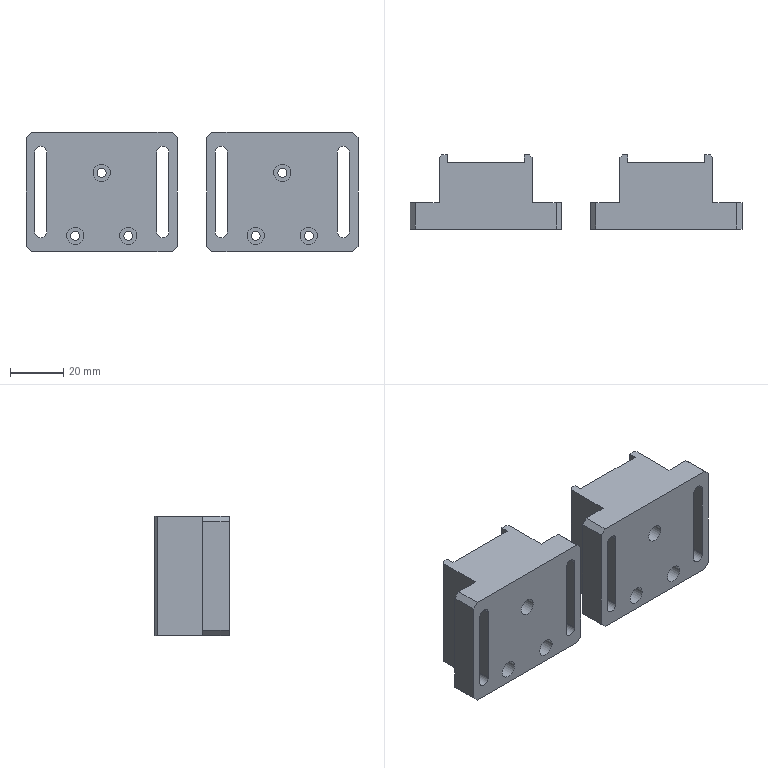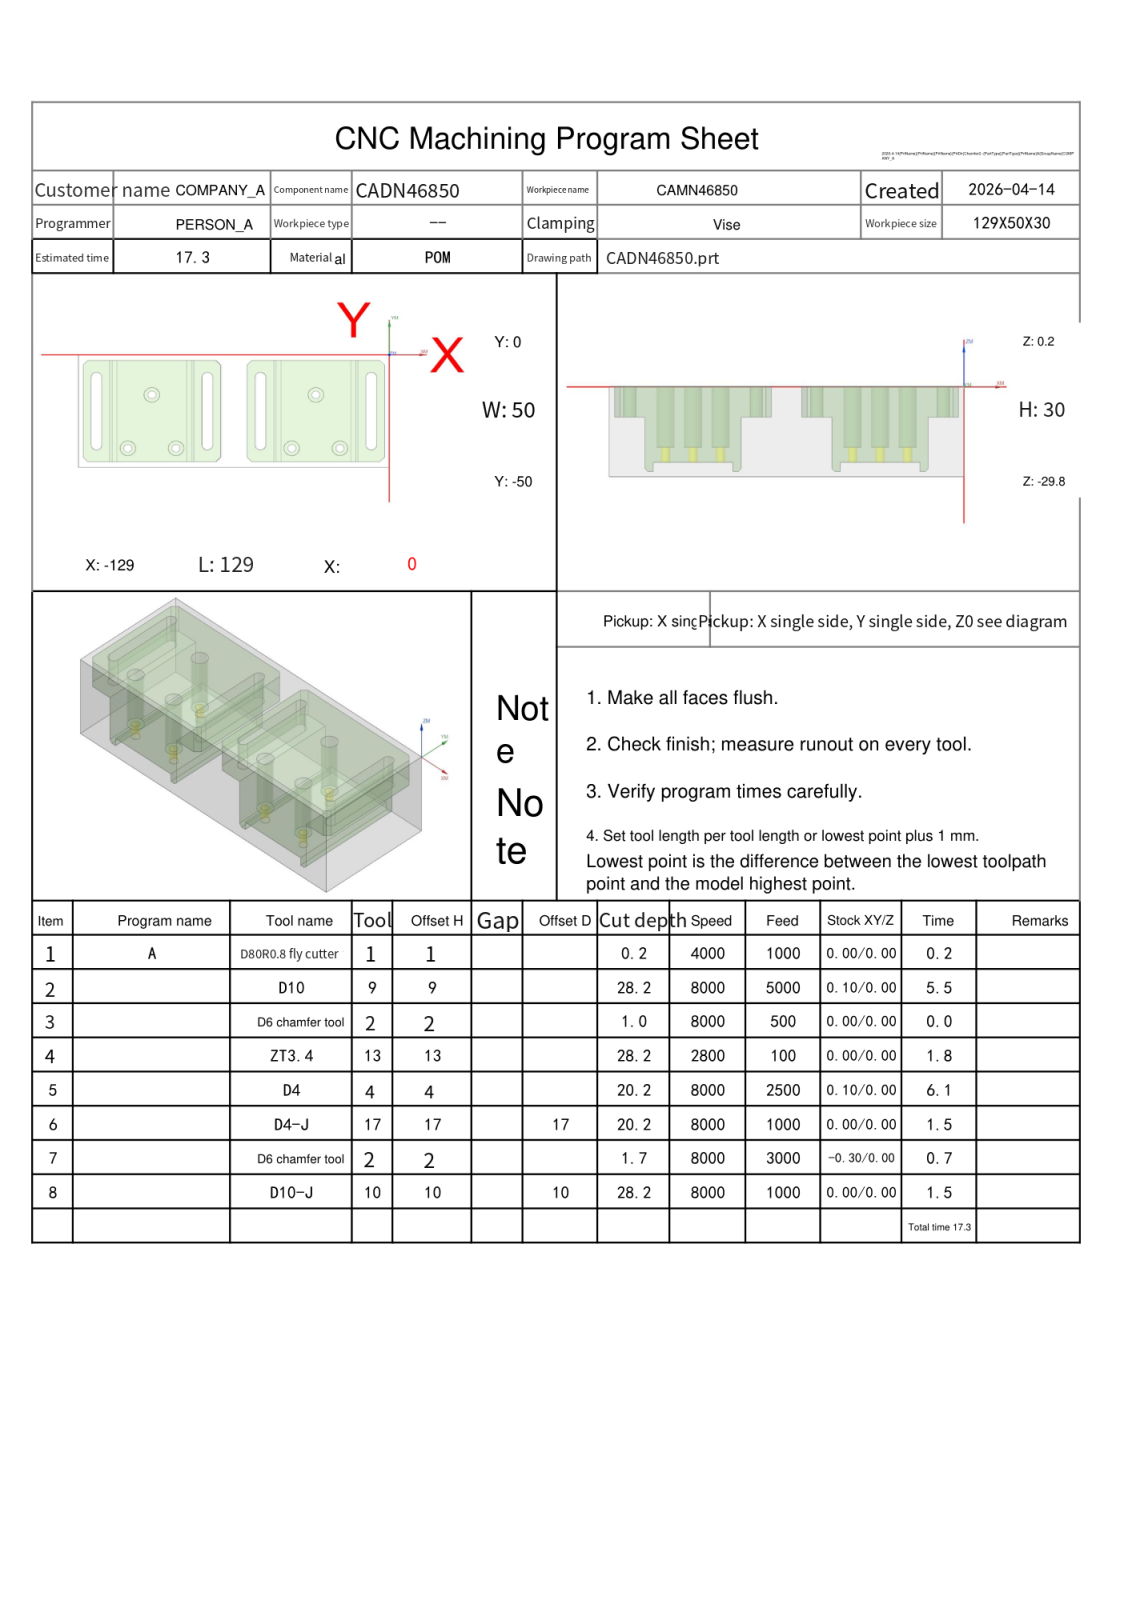NC program | NX | posted by the shop | part box 125 x 28 x 45 mm
Lines 1997 to 3630 of 4607, first 1124 of 1634 lines:
N5 T04 M06
(D4  D=4. R=0. H=04 ce=0.10 di=0.10)
G00 G90 G54 X-7.65 Y-25. M03 S6000
G43 H04 Z20.
M08
Z.5
G01 Y-40. Z.44 F2500.
G03 X-7.5 Y-40.15 Z.439 I.15 J0.0
X-7.35 Y-40. Z.438 I0.0 J.15
G01 Y-10. Z.318
G03 X-7.5 Y-9.85 Z.317 I-.15 J0.0
X-7.65 Y-10. Z.316 I0.0 J-.15
G01 Y-40. Z.195
G03 X-7.5 Y-40.15 Z.194 I.15 J0.0
X-7.35 Y-40. Z.194 I0.0 J.15
G01 Y-10. Z.073
G03 X-7.5 Y-9.85 Z.072 I-.15 J0.0
X-7.65 Y-10. Z.071 I0.0 J-.15
G01 Y-40. Z-.049
G03 X-7.5 Y-40.15 Z-.05 I.15 J0.0
X-7.35 Y-40. Z-.051 I0.0 J.15
G01 Y-10. Z-.171
G03 X-7.5 Y-9.85 Z-.172 I-.15 J0.0
X-7.65 Y-10. Z-.173 I0.0 J-.15
G01 Y-40. Z-.294
G03 X-7.5 Y-40.15 Z-.294 I.15 J0.0
X-7.35 Y-40. Z-.295 I0.0 J.15
G01 Y-10. Z-.416
G03 X-7.5 Y-9.85 Z-.417 I-.15 J0.0
X-7.65 Y-10. Z-.418 I0.0 J-.15
G01 Y-40. Z-.538
G03 X-7.5 Y-40.15 Z-.539 I.15 J0.0
X-7.35 Y-40. Z-.54 I0.0 J.15
G01 Y-10. Z-.66
G03 X-7.5 Y-9.85 Z-.661 I-.15 J0.0
X-7.65 Y-10. Z-.662 I0.0 J-.15
G01 Y-40. Z-.782
G03 X-7.5 Y-40.15 Z-.783 I.15 J0.0
X-7.35 Y-40. Z-.784 I0.0 J.15
G01 Y-10. Z-.905
G03 X-7.5 Y-9.85 Z-.906 I-.15 J0.0
X-7.65 Y-10. Z-.907 I0.0 J-.15
G01 Y-40. Z-1.027
G03 X-7.5 Y-40.15 Z-1.028 I.15 J0.0
X-7.35 Y-40. Z-1.029 I0.0 J.15
G01 Y-10. Z-1.149
G03 X-7.5 Y-9.85 Z-1.15 I-.15 J0.0
X-7.65 Y-10. Z-1.151 I0.0 J-.15
G01 Y-40. Z-1.271
G03 X-7.5 Y-40.15 Z-1.272 I.15 J0.0
X-7.35 Y-40. Z-1.273 I0.0 J.15
G01 Y-10. Z-1.394
G03 X-7.5 Y-9.85 Z-1.394 I-.15 J0.0
X-7.65 Y-10. Z-1.395 I0.0 J-.15
G01 Y-40. Z-1.516
G03 X-7.5 Y-40.15 Z-1.517 I.15 J0.0
X-7.35 Y-40. Z-1.518 I0.0 J.15
G01 Y-10. Z-1.638
G03 X-7.5 Y-9.85 Z-1.639 I-.15 J0.0
X-7.65 Y-10. Z-1.64 I0.0 J-.15
G01 Y-40. Z-1.76
G03 X-7.5 Y-40.15 Z-1.761 I.15 J0.0
X-7.35 Y-40. Z-1.762 I0.0 J.15
G01 Y-10. Z-1.882
G03 X-7.5 Y-9.85 Z-1.883 I-.15 J0.0
X-7.65 Y-10. Z-1.884 I0.0 J-.15
G01 Y-40. Z-2.005
G03 X-7.5 Y-40.15 Z-2.006 I.15 J0.0
X-7.35 Y-40. Z-2.007 I0.0 J.15
G01 Y-10. Z-2.127
G03 X-7.5 Y-9.85 Z-2.128 I-.15 J0.0
X-7.65 Y-10. Z-2.129 I0.0 J-.15
G01 Y-40. Z-2.249
G03 X-7.5 Y-40.15 Z-2.25 I.15 J0.0
X-7.35 Y-40. Z-2.251 I0.0 J.15
G01 Y-10. Z-2.371
G03 X-7.5 Y-9.85 Z-2.372 I-.15 J0.0
X-7.65 Y-10. Z-2.373 I0.0 J-.15
G01 Y-40. Z-2.494
G03 X-7.5 Y-40.15 Z-2.494 I.15 J0.0
X-7.35 Y-40. Z-2.495 I0.0 J.15
G01 Y-10. Z-2.616
G03 X-7.5 Y-9.85 Z-2.617 I-.15 J0.0
X-7.65 Y-10. Z-2.618 I0.0 J-.15
G01 Y-40. Z-2.738
G03 X-7.5 Y-40.15 Z-2.739 I.15 J0.0
X-7.35 Y-40. Z-2.74 I0.0 J.15
G01 Y-10. Z-2.86
G03 X-7.5 Y-9.85 Z-2.861 I-.15 J0.0
X-7.65 Y-10. Z-2.862 I0.0 J-.15
G01 Y-40. Z-2.982
G03 X-7.5 Y-40.15 Z-2.983 I.15 J0.0
X-7.35 Y-40. Z-2.984 I0.0 J.15
G01 Y-10. Z-3.105
G03 X-7.5 Y-9.85 Z-3.106 I-.15 J0.0
X-7.65 Y-10. Z-3.107 I0.0 J-.15
G01 Y-40. Z-3.227
G03 X-7.5 Y-40.15 Z-3.228 I.15 J0.0
X-7.35 Y-40. Z-3.229 I0.0 J.15
G01 Y-10. Z-3.349
G03 X-7.5 Y-9.85 Z-3.35 I-.15 J0.0
X-7.65 Y-10. Z-3.351 I0.0 J-.15
G01 Y-40. Z-3.471
G03 X-7.5 Y-40.15 Z-3.472 I.15 J0.0
X-7.35 Y-40. Z-3.473 I0.0 J.15
G01 Y-10. Z-3.594
G03 X-7.5 Y-9.85 Z-3.594 I-.15 J0.0
X-7.65 Y-10. Z-3.595 I0.0 J-.15
G01 Y-40. Z-3.716
G03 X-7.5 Y-40.15 Z-3.717 I.15 J0.0
X-7.35 Y-40. Z-3.718 I0.0 J.15
G01 Y-10. Z-3.838
G03 X-7.5 Y-9.85 Z-3.839 I-.15 J0.0
X-7.65 Y-10. Z-3.84 I0.0 J-.15
G01 Y-40. Z-3.96
G03 X-7.5 Y-40.15 Z-3.961 I.15 J0.0
X-7.35 Y-40. Z-3.962 I0.0 J.15
G01 Y-10. Z-4.082
G03 X-7.5 Y-9.85 Z-4.083 I-.15 J0.0
X-7.65 Y-10. Z-4.084 I0.0 J-.15
G01 Y-40. Z-4.205
G03 X-7.5 Y-40.15 Z-4.206 I.15 J0.0
X-7.35 Y-40. Z-4.207 I0.0 J.15
G01 Y-10. Z-4.327
G03 X-7.5 Y-9.85 Z-4.328 I-.15 J0.0
X-7.65 Y-10. Z-4.329 I0.0 J-.15
G01 Y-40. Z-4.449
G03 X-7.5 Y-40.15 Z-4.45 I.15 J0.0
X-7.35 Y-40. Z-4.451 I0.0 J.15
G01 Y-10. Z-4.571
G03 X-7.5 Y-9.85 Z-4.572 I-.15 J0.0
X-7.65 Y-10. Z-4.573 I0.0 J-.15
G01 Y-40. Z-4.694
G03 X-7.5 Y-40.15 Z-4.694 I.15 J0.0
X-7.35 Y-40. Z-4.695 I0.0 J.15
G01 Y-10. Z-4.816
G03 X-7.5 Y-9.85 Z-4.817 I-.15 J0.0
X-7.65 Y-10. Z-4.818 I0.0 J-.15
G01 Y-40. Z-4.938
G03 X-7.5 Y-40.15 Z-4.939 I.15 J0.0
X-7.35 Y-40. Z-4.94 I0.0 J.15
G01 Y-10. Z-5.06
G03 X-7.5 Y-9.85 Z-5.061 I-.15 J0.0
X-7.65 Y-10. Z-5.062 I0.0 J-.15
G01 Y-40. Z-5.182
G03 X-7.5 Y-40.15 Z-5.183 I.15 J0.0
X-7.35 Y-40. Z-5.184 I0.0 J.15
G01 Y-10. Z-5.305
G03 X-7.5 Y-9.85 Z-5.306 I-.15 J0.0
X-7.65 Y-10. Z-5.307 I0.0 J-.15
G01 Y-40. Z-5.427
G03 X-7.5 Y-40.15 Z-5.428 I.15 J0.0
X-7.35 Y-40. Z-5.429 I0.0 J.15
G01 Y-10. Z-5.549
G03 X-7.5 Y-9.85 Z-5.55 I-.15 J0.0
X-7.65 Y-10. Z-5.551 I0.0 J-.15
G01 Y-40. Z-5.671
G03 X-7.5 Y-40.15 Z-5.672 I.15 J0.0
X-7.35 Y-40. Z-5.673 I0.0 J.15
G01 Y-10. Z-5.794
G03 X-7.5 Y-9.85 Z-5.794 I-.15 J0.0
X-7.65 Y-10. Z-5.795 I0.0 J-.15
G01 Y-40. Z-5.916
G03 X-7.5 Y-40.15 Z-5.917 I.15 J0.0
X-7.35 Y-40. Z-5.918 I0.0 J.15
G01 Y-10. Z-6.038
G03 X-7.5 Y-9.85 Z-6.039 I-.15 J0.0
X-7.65 Y-10. Z-6.04 I0.0 J-.15
G01 Y-40. Z-6.16
G03 X-7.5 Y-40.15 Z-6.161 I.15 J0.0
X-7.35 Y-40. Z-6.162 I0.0 J.15
G01 Y-10. Z-6.282
G03 X-7.5 Y-9.85 Z-6.283 I-.15 J0.0
X-7.65 Y-10. Z-6.284 I0.0 J-.15
G01 Y-40. Z-6.405
G03 X-7.5 Y-40.15 Z-6.406 I.15 J0.0
X-7.35 Y-40. Z-6.407 I0.0 J.15
G01 Y-10. Z-6.527
G03 X-7.5 Y-9.85 Z-6.528 I-.15 J0.0
X-7.65 Y-10. Z-6.529 I0.0 J-.15
G01 Y-40. Z-6.649
G03 X-7.5 Y-40.15 Z-6.65 I.15 J0.0
X-7.35 Y-40. Z-6.651 I0.0 J.15
G01 Y-10. Z-6.771
G03 X-7.5 Y-9.85 Z-6.772 I-.15 J0.0
X-7.65 Y-10. Z-6.773 I0.0 J-.15
G01 Y-40. Z-6.894
G03 X-7.5 Y-40.15 Z-6.894 I.15 J0.0
X-7.35 Y-40. Z-6.895 I0.0 J.15
G01 Y-10. Z-7.016
G03 X-7.5 Y-9.85 Z-7.017 I-.15 J0.0
X-7.65 Y-10. Z-7.018 I0.0 J-.15
G01 Y-40. Z-7.138
G03 X-7.5 Y-40.15 Z-7.139 I.15 J0.0
X-7.35 Y-40. Z-7.14 I0.0 J.15
G01 Y-10. Z-7.26
G03 X-7.5 Y-9.85 Z-7.261 I-.15 J0.0
X-7.65 Y-10. Z-7.262 I0.0 J-.15
G01 Y-40. Z-7.382
G03 X-7.5 Y-40.15 Z-7.383 I.15 J0.0
X-7.35 Y-40. Z-7.384 I0.0 J.15
G01 Y-10. Z-7.505
G03 X-7.5 Y-9.85 Z-7.506 I-.15 J0.0
X-7.65 Y-10. Z-7.507 I0.0 J-.15
G01 Y-40. Z-7.627
G03 X-7.5 Y-40.15 Z-7.628 I.15 J0.0
X-7.35 Y-40. Z-7.629 I0.0 J.15
G01 Y-10. Z-7.749
G03 X-7.5 Y-9.85 Z-7.75 I-.15 J0.0
X-7.65 Y-10. Z-7.751 I0.0 J-.15
G01 Y-40. Z-7.871
G03 X-7.5 Y-40.15 Z-7.872 I.15 J0.0
X-7.35 Y-40. Z-7.873 I0.0 J.15
G01 Y-10. Z-7.994
G03 X-7.5 Y-9.85 Z-7.994 I-.15 J0.0
X-7.65 Y-10. Z-7.995 I0.0 J-.15
G01 Y-40. Z-8.116
G03 X-7.5 Y-40.15 Z-8.117 I.15 J0.0
X-7.35 Y-40. Z-8.118 I0.0 J.15
G01 Y-10. Z-8.238
G03 X-7.5 Y-9.85 Z-8.239 I-.15 J0.0
X-7.65 Y-10. Z-8.24 I0.0 J-.15
G01 Y-40. Z-8.36
G03 X-7.5 Y-40.15 Z-8.361 I.15 J0.0
X-7.35 Y-40. Z-8.362 I0.0 J.15
G01 Y-10. Z-8.482
G03 X-7.5 Y-9.85 Z-8.483 I-.15 J0.0
X-7.65 Y-10. Z-8.484 I0.0 J-.15
G01 Y-40. Z-8.605
G03 X-7.5 Y-40.15 Z-8.606 I.15 J0.0
X-7.35 Y-40. Z-8.607 I0.0 J.15
G01 Y-10. Z-8.727
G03 X-7.5 Y-9.85 Z-8.728 I-.15 J0.0
X-7.65 Y-10. Z-8.729 I0.0 J-.15
G01 Y-40. Z-8.849
G03 X-7.5 Y-40.15 Z-8.85 I.15 J0.0
X-7.35 Y-40. Z-8.851 I0.0 J.15
G01 Y-10. Z-8.971
G03 X-7.5 Y-9.85 Z-8.972 I-.15 J0.0
X-7.65 Y-10. Z-8.973 I0.0 J-.15
G01 Y-40. Z-9.094
G03 X-7.5 Y-40.15 Z-9.094 I.15 J0.0
X-7.35 Y-40. Z-9.095 I0.0 J.15
G01 Y-10. Z-9.216
G03 X-7.5 Y-9.85 Z-9.217 I-.15 J0.0
X-7.65 Y-10. Z-9.218 I0.0 J-.15
G01 Y-40. Z-9.338
G03 X-7.5 Y-40.15 Z-9.339 I.15 J0.0
X-7.35 Y-40. Z-9.34 I0.0 J.15
G01 Y-10. Z-9.46
G03 X-7.5 Y-9.85 Z-9.461 I-.15 J0.0
X-7.65 Y-10. Z-9.462 I0.0 J-.15
G01 Y-40. Z-9.582
G03 X-7.5 Y-40.15 Z-9.583 I.15 J0.0
X-7.35 Y-40. Z-9.584 I0.0 J.15
G01 Y-10. Z-9.705
G03 X-7.5 Y-9.85 Z-9.706 I-.15 J0.0
X-7.65 Y-10. Z-9.707 I0.0 J-.15
G01 Y-40. Z-9.827
G03 X-7.5 Y-40.15 Z-9.828 I.15 J0.0
X-7.35 Y-40. Z-9.829 I0.0 J.15
G01 Y-10. Z-9.949
G03 X-7.5 Y-9.85 Z-9.95 I-.15 J0.0
X-7.65 Y-10. Z-9.951 I0.0 J-.15
G01 Y-40. Z-10.071
G03 X-7.5 Y-40.15 Z-10.072 I.15 J0.0
X-7.35 Y-40. Z-10.073 I0.0 J.15
G01 Y-10. Z-10.194
G03 X-7.5 Y-9.85 Z-10.194 I-.15 J0.0
X-7.65 Y-10. Z-10.195 I0.0 J-.15
G01 Y-40. Z-10.316
G03 X-7.5 Y-40.15 Z-10.317 I.15 J0.0
X-7.35 Y-40. Z-10.318 I0.0 J.15
G01 Y-10. Z-10.438
G03 X-7.5 Y-9.85 Z-10.439 I-.15 J0.0
X-7.65 Y-10. Z-10.44 I0.0 J-.15
G01 Y-25. Z-10.5
Y-40.
G03 X-7.5 Y-40.15 I.15 J0.0
X-7.35 Y-40. I0.0 J.15
G01 Y-10.
G03 X-7.5 Y-9.85 I-.15 J0.0
X-7.65 Y-10. I0.0 J-.15
G01 Y-25.
Y-25.5
Z-9.5
G00 Z20.
X-53.35 Y-25.
Z.5
G01 Y-10. Z.44
G03 X-53.5 Y-9.85 Z.439 I-.15 J0.0
X-53.65 Y-10. Z.438 I0.0 J-.15
G01 Y-40. Z.318
G03 X-53.5 Y-40.15 Z.317 I.15 J0.0
X-53.35 Y-40. Z.316 I0.0 J.15
G01 Y-10. Z.195
G03 X-53.5 Y-9.85 Z.194 I-.15 J0.0
X-53.65 Y-10. Z.194 I0.0 J-.15
G01 Y-40. Z.073
G03 X-53.5 Y-40.15 Z.072 I.15 J0.0
X-53.35 Y-40. Z.071 I0.0 J.15
G01 Y-10. Z-.049
G03 X-53.5 Y-9.85 Z-.05 I-.15 J0.0
X-53.65 Y-10. Z-.051 I0.0 J-.15
G01 Y-40. Z-.171
G03 X-53.5 Y-40.15 Z-.172 I.15 J0.0
X-53.35 Y-40. Z-.173 I0.0 J.15
G01 Y-10. Z-.294
G03 X-53.5 Y-9.85 Z-.294 I-.15 J0.0
X-53.65 Y-10. Z-.295 I0.0 J-.15
G01 Y-40. Z-.416
G03 X-53.5 Y-40.15 Z-.417 I.15 J0.0
X-53.35 Y-40. Z-.418 I0.0 J.15
G01 Y-10. Z-.538
G03 X-53.5 Y-9.85 Z-.539 I-.15 J0.0
X-53.65 Y-10. Z-.54 I0.0 J-.15
G01 Y-40. Z-.66
G03 X-53.5 Y-40.15 Z-.661 I.15 J0.0
X-53.35 Y-40. Z-.662 I0.0 J.15
G01 Y-10. Z-.782
G03 X-53.5 Y-9.85 Z-.783 I-.15 J0.0
X-53.65 Y-10. Z-.784 I0.0 J-.15
G01 Y-40. Z-.905
G03 X-53.5 Y-40.15 Z-.906 I.15 J0.0
X-53.35 Y-40. Z-.907 I0.0 J.15
G01 Y-10. Z-1.027
G03 X-53.5 Y-9.85 Z-1.028 I-.15 J0.0
X-53.65 Y-10. Z-1.029 I0.0 J-.15
G01 Y-40. Z-1.149
G03 X-53.5 Y-40.15 Z-1.15 I.15 J0.0
X-53.35 Y-40. Z-1.151 I0.0 J.15
G01 Y-10. Z-1.271
G03 X-53.5 Y-9.85 Z-1.272 I-.15 J0.0
X-53.65 Y-10. Z-1.273 I0.0 J-.15
G01 Y-40. Z-1.394
G03 X-53.5 Y-40.15 Z-1.394 I.15 J0.0
X-53.35 Y-40. Z-1.395 I0.0 J.15
G01 Y-10. Z-1.516
G03 X-53.5 Y-9.85 Z-1.517 I-.15 J0.0
X-53.65 Y-10. Z-1.518 I0.0 J-.15
G01 Y-40. Z-1.638
G03 X-53.5 Y-40.15 Z-1.639 I.15 J0.0
X-53.35 Y-40. Z-1.64 I0.0 J.15
G01 Y-10. Z-1.76
G03 X-53.5 Y-9.85 Z-1.761 I-.15 J0.0
X-53.65 Y-10. Z-1.762 I0.0 J-.15
G01 Y-40. Z-1.882
G03 X-53.5 Y-40.15 Z-1.883 I.15 J0.0
X-53.35 Y-40. Z-1.884 I0.0 J.15
G01 Y-10. Z-2.005
G03 X-53.5 Y-9.85 Z-2.006 I-.15 J0.0
X-53.65 Y-10. Z-2.007 I0.0 J-.15
G01 Y-40. Z-2.127
G03 X-53.5 Y-40.15 Z-2.128 I.15 J0.0
X-53.35 Y-40. Z-2.129 I0.0 J.15
G01 Y-10. Z-2.249
G03 X-53.5 Y-9.85 Z-2.25 I-.15 J0.0
X-53.65 Y-10. Z-2.251 I0.0 J-.15
G01 Y-40. Z-2.371
G03 X-53.5 Y-40.15 Z-2.372 I.15 J0.0
X-53.35 Y-40. Z-2.373 I0.0 J.15
G01 Y-10. Z-2.494
G03 X-53.5 Y-9.85 Z-2.494 I-.15 J0.0
X-53.65 Y-10. Z-2.495 I0.0 J-.15
G01 Y-40. Z-2.616
G03 X-53.5 Y-40.15 Z-2.617 I.15 J0.0
X-53.35 Y-40. Z-2.618 I0.0 J.15
G01 Y-10. Z-2.738
G03 X-53.5 Y-9.85 Z-2.739 I-.15 J0.0
X-53.65 Y-10. Z-2.74 I0.0 J-.15
G01 Y-40. Z-2.86
G03 X-53.5 Y-40.15 Z-2.861 I.15 J0.0
X-53.35 Y-40. Z-2.862 I0.0 J.15
G01 Y-10. Z-2.982
G03 X-53.5 Y-9.85 Z-2.983 I-.15 J0.0
X-53.65 Y-10. Z-2.984 I0.0 J-.15
G01 Y-40. Z-3.105
G03 X-53.5 Y-40.15 Z-3.106 I.15 J0.0
X-53.35 Y-40. Z-3.107 I0.0 J.15
G01 Y-10. Z-3.227
G03 X-53.5 Y-9.85 Z-3.228 I-.15 J0.0
X-53.65 Y-10. Z-3.229 I0.0 J-.15
G01 Y-40. Z-3.349
G03 X-53.5 Y-40.15 Z-3.35 I.15 J0.0
X-53.35 Y-40. Z-3.351 I0.0 J.15
G01 Y-10. Z-3.471
G03 X-53.5 Y-9.85 Z-3.472 I-.15 J0.0
X-53.65 Y-10. Z-3.473 I0.0 J-.15
G01 Y-40. Z-3.594
G03 X-53.5 Y-40.15 Z-3.594 I.15 J0.0
X-53.35 Y-40. Z-3.595 I0.0 J.15
G01 Y-10. Z-3.716
G03 X-53.5 Y-9.85 Z-3.717 I-.15 J0.0
X-53.65 Y-10. Z-3.718 I0.0 J-.15
G01 Y-40. Z-3.838
G03 X-53.5 Y-40.15 Z-3.839 I.15 J0.0
X-53.35 Y-40. Z-3.84 I0.0 J.15
G01 Y-10. Z-3.96
G03 X-53.5 Y-9.85 Z-3.961 I-.15 J0.0
X-53.65 Y-10. Z-3.962 I0.0 J-.15
G01 Y-40. Z-4.082
G03 X-53.5 Y-40.15 Z-4.083 I.15 J0.0
X-53.35 Y-40. Z-4.084 I0.0 J.15
G01 Y-10. Z-4.205
G03 X-53.5 Y-9.85 Z-4.206 I-.15 J0.0
X-53.65 Y-10. Z-4.207 I0.0 J-.15
G01 Y-40. Z-4.327
G03 X-53.5 Y-40.15 Z-4.328 I.15 J0.0
X-53.35 Y-40. Z-4.329 I0.0 J.15
G01 Y-10. Z-4.449
G03 X-53.5 Y-9.85 Z-4.45 I-.15 J0.0
X-53.65 Y-10. Z-4.451 I0.0 J-.15
G01 Y-40. Z-4.571
G03 X-53.5 Y-40.15 Z-4.572 I.15 J0.0
X-53.35 Y-40. Z-4.573 I0.0 J.15
G01 Y-10. Z-4.694
G03 X-53.5 Y-9.85 Z-4.694 I-.15 J0.0
X-53.65 Y-10. Z-4.695 I0.0 J-.15
G01 Y-40. Z-4.816
G03 X-53.5 Y-40.15 Z-4.817 I.15 J0.0
X-53.35 Y-40. Z-4.818 I0.0 J.15
G01 Y-10. Z-4.938
G03 X-53.5 Y-9.85 Z-4.939 I-.15 J0.0
X-53.65 Y-10. Z-4.94 I0.0 J-.15
G01 Y-40. Z-5.06
G03 X-53.5 Y-40.15 Z-5.061 I.15 J0.0
X-53.35 Y-40. Z-5.062 I0.0 J.15
G01 Y-10. Z-5.182
G03 X-53.5 Y-9.85 Z-5.183 I-.15 J0.0
X-53.65 Y-10. Z-5.184 I0.0 J-.15
G01 Y-40. Z-5.305
G03 X-53.5 Y-40.15 Z-5.306 I.15 J0.0
X-53.35 Y-40. Z-5.307 I0.0 J.15
G01 Y-10. Z-5.427
G03 X-53.5 Y-9.85 Z-5.428 I-.15 J0.0
X-53.65 Y-10. Z-5.429 I0.0 J-.15
G01 Y-40. Z-5.549
G03 X-53.5 Y-40.15 Z-5.55 I.15 J0.0
X-53.35 Y-40. Z-5.551 I0.0 J.15
G01 Y-10. Z-5.671
G03 X-53.5 Y-9.85 Z-5.672 I-.15 J0.0
X-53.65 Y-10. Z-5.673 I0.0 J-.15
G01 Y-40. Z-5.794
G03 X-53.5 Y-40.15 Z-5.794 I.15 J0.0
X-53.35 Y-40. Z-5.795 I0.0 J.15
G01 Y-10. Z-5.916
G03 X-53.5 Y-9.85 Z-5.917 I-.15 J0.0
X-53.65 Y-10. Z-5.918 I0.0 J-.15
G01 Y-40. Z-6.038
G03 X-53.5 Y-40.15 Z-6.039 I.15 J0.0
X-53.35 Y-40. Z-6.04 I0.0 J.15
G01 Y-10. Z-6.16
G03 X-53.5 Y-9.85 Z-6.161 I-.15 J0.0
X-53.65 Y-10. Z-6.162 I0.0 J-.15
G01 Y-40. Z-6.282
G03 X-53.5 Y-40.15 Z-6.283 I.15 J0.0
X-53.35 Y-40. Z-6.284 I0.0 J.15
G01 Y-10. Z-6.405
G03 X-53.5 Y-9.85 Z-6.406 I-.15 J0.0
X-53.65 Y-10. Z-6.407 I0.0 J-.15
G01 Y-40. Z-6.527
G03 X-53.5 Y-40.15 Z-6.528 I.15 J0.0
X-53.35 Y-40. Z-6.529 I0.0 J.15
G01 Y-10. Z-6.649
G03 X-53.5 Y-9.85 Z-6.65 I-.15 J0.0
X-53.65 Y-10. Z-6.651 I0.0 J-.15
G01 Y-40. Z-6.771
G03 X-53.5 Y-40.15 Z-6.772 I.15 J0.0
X-53.35 Y-40. Z-6.773 I0.0 J.15
G01 Y-10. Z-6.894
G03 X-53.5 Y-9.85 Z-6.894 I-.15 J0.0
X-53.65 Y-10. Z-6.895 I0.0 J-.15
G01 Y-40. Z-7.016
G03 X-53.5 Y-40.15 Z-7.017 I.15 J0.0
X-53.35 Y-40. Z-7.018 I0.0 J.15
G01 Y-10. Z-7.138
G03 X-53.5 Y-9.85 Z-7.139 I-.15 J0.0
X-53.65 Y-10. Z-7.14 I0.0 J-.15
G01 Y-40. Z-7.26
G03 X-53.5 Y-40.15 Z-7.261 I.15 J0.0
X-53.35 Y-40. Z-7.262 I0.0 J.15
G01 Y-10. Z-7.382
G03 X-53.5 Y-9.85 Z-7.383 I-.15 J0.0
X-53.65 Y-10. Z-7.384 I0.0 J-.15
G01 Y-40. Z-7.505
G03 X-53.5 Y-40.15 Z-7.506 I.15 J0.0
X-53.35 Y-40. Z-7.507 I0.0 J.15
G01 Y-10. Z-7.627
G03 X-53.5 Y-9.85 Z-7.628 I-.15 J0.0
X-53.65 Y-10. Z-7.629 I0.0 J-.15
G01 Y-40. Z-7.749
G03 X-53.5 Y-40.15 Z-7.75 I.15 J0.0
X-53.35 Y-40. Z-7.751 I0.0 J.15
G01 Y-10. Z-7.871
G03 X-53.5 Y-9.85 Z-7.872 I-.15 J0.0
X-53.65 Y-10. Z-7.873 I0.0 J-.15
G01 Y-40. Z-7.994
G03 X-53.5 Y-40.15 Z-7.994 I.15 J0.0
X-53.35 Y-40. Z-7.995 I0.0 J.15
G01 Y-10. Z-8.116
G03 X-53.5 Y-9.85 Z-8.117 I-.15 J0.0
X-53.65 Y-10. Z-8.118 I0.0 J-.15
G01 Y-40. Z-8.238
G03 X-53.5 Y-40.15 Z-8.239 I.15 J0.0
X-53.35 Y-40. Z-8.24 I0.0 J.15
G01 Y-10. Z-8.36
G03 X-53.5 Y-9.85 Z-8.361 I-.15 J0.0
X-53.65 Y-10. Z-8.362 I0.0 J-.15
G01 Y-40. Z-8.482
G03 X-53.5 Y-40.15 Z-8.483 I.15 J0.0
X-53.35 Y-40. Z-8.484 I0.0 J.15
G01 Y-10. Z-8.605
G03 X-53.5 Y-9.85 Z-8.606 I-.15 J0.0
X-53.65 Y-10. Z-8.607 I0.0 J-.15
G01 Y-40. Z-8.727
G03 X-53.5 Y-40.15 Z-8.728 I.15 J0.0
X-53.35 Y-40. Z-8.729 I0.0 J.15
G01 Y-10. Z-8.849
G03 X-53.5 Y-9.85 Z-8.85 I-.15 J0.0
X-53.65 Y-10. Z-8.851 I0.0 J-.15
G01 Y-40. Z-8.971
G03 X-53.5 Y-40.15 Z-8.972 I.15 J0.0
X-53.35 Y-40. Z-8.973 I0.0 J.15
G01 Y-10. Z-9.094
G03 X-53.5 Y-9.85 Z-9.094 I-.15 J0.0
X-53.65 Y-10. Z-9.095 I0.0 J-.15
G01 Y-40. Z-9.216
G03 X-53.5 Y-40.15 Z-9.217 I.15 J0.0
X-53.35 Y-40. Z-9.218 I0.0 J.15
G01 Y-10. Z-9.338
G03 X-53.5 Y-9.85 Z-9.339 I-.15 J0.0
X-53.65 Y-10. Z-9.34 I0.0 J-.15
G01 Y-40. Z-9.46
G03 X-53.5 Y-40.15 Z-9.461 I.15 J0.0
X-53.35 Y-40. Z-9.462 I0.0 J.15
G01 Y-10. Z-9.582
G03 X-53.5 Y-9.85 Z-9.583 I-.15 J0.0
X-53.65 Y-10. Z-9.584 I0.0 J-.15
G01 Y-40. Z-9.705
G03 X-53.5 Y-40.15 Z-9.706 I.15 J0.0
X-53.35 Y-40. Z-9.707 I0.0 J.15
G01 Y-10. Z-9.827
G03 X-53.5 Y-9.85 Z-9.828 I-.15 J0.0
X-53.65 Y-10. Z-9.829 I0.0 J-.15
G01 Y-40. Z-9.949
G03 X-53.5 Y-40.15 Z-9.95 I.15 J0.0
X-53.35 Y-40. Z-9.951 I0.0 J.15
G01 Y-10. Z-10.071
G03 X-53.5 Y-9.85 Z-10.072 I-.15 J0.0
X-53.65 Y-10. Z-10.073 I0.0 J-.15
G01 Y-40. Z-10.194
G03 X-53.5 Y-40.15 Z-10.194 I.15 J0.0
X-53.35 Y-40. Z-10.195 I0.0 J.15
G01 Y-10. Z-10.316
G03 X-53.5 Y-9.85 Z-10.317 I-.15 J0.0
X-53.65 Y-10. Z-10.318 I0.0 J-.15
G01 Y-40. Z-10.438
G03 X-53.5 Y-40.15 Z-10.439 I.15 J0.0
X-53.35 Y-40. Z-10.44 I0.0 J.15
G01 Y-25. Z-10.5
Y-10.
G03 X-53.5 Y-9.85 I-.15 J0.0
X-53.65 Y-10. I0.0 J-.15
G01 Y-40.
G03 X-53.5 Y-40.15 I.15 J0.0
X-53.35 Y-40. I0.0 J.15
G01 Y-25.
Y-24.5
Z-9.5
G00 Z20.
X-75.35 Y-25.
Z.5
G01 Y-10. Z.44
G03 X-75.5 Y-9.85 Z.439 I-.15 J0.0
X-75.65 Y-10. Z.438 I0.0 J-.15
G01 Y-40. Z.318
G03 X-75.5 Y-40.15 Z.317 I.15 J0.0
X-75.35 Y-40. Z.316 I0.0 J.15
G01 Y-10. Z.195
G03 X-75.5 Y-9.85 Z.194 I-.15 J0.0
X-75.65 Y-10. Z.194 I0.0 J-.15
G01 Y-40. Z.073
G03 X-75.5 Y-40.15 Z.072 I.15 J0.0
X-75.35 Y-40. Z.071 I0.0 J.15
G01 Y-10. Z-.049
G03 X-75.5 Y-9.85 Z-.05 I-.15 J0.0
X-75.65 Y-10. Z-.051 I0.0 J-.15
G01 Y-40. Z-.171
G03 X-75.5 Y-40.15 Z-.172 I.15 J0.0
X-75.35 Y-40. Z-.173 I0.0 J.15
G01 Y-10. Z-.294
G03 X-75.5 Y-9.85 Z-.294 I-.15 J0.0
X-75.65 Y-10. Z-.295 I0.0 J-.15
G01 Y-40. Z-.416
G03 X-75.5 Y-40.15 Z-.417 I.15 J0.0
X-75.35 Y-40. Z-.418 I0.0 J.15
G01 Y-10. Z-.538
G03 X-75.5 Y-9.85 Z-.539 I-.15 J0.0
X-75.65 Y-10. Z-.54 I0.0 J-.15
G01 Y-40. Z-.66
G03 X-75.5 Y-40.15 Z-.661 I.15 J0.0
X-75.35 Y-40. Z-.662 I0.0 J.15
G01 Y-10. Z-.782
G03 X-75.5 Y-9.85 Z-.783 I-.15 J0.0
X-75.65 Y-10. Z-.784 I0.0 J-.15
G01 Y-40. Z-.905
G03 X-75.5 Y-40.15 Z-.906 I.15 J0.0
X-75.35 Y-40. Z-.907 I0.0 J.15
G01 Y-10. Z-1.027
G03 X-75.5 Y-9.85 Z-1.028 I-.15 J0.0
X-75.65 Y-10. Z-1.029 I0.0 J-.15
G01 Y-40. Z-1.149
G03 X-75.5 Y-40.15 Z-1.15 I.15 J0.0
X-75.35 Y-40. Z-1.151 I0.0 J.15
G01 Y-10. Z-1.271
G03 X-75.5 Y-9.85 Z-1.272 I-.15 J0.0
X-75.65 Y-10. Z-1.273 I0.0 J-.15
G01 Y-40. Z-1.394
G03 X-75.5 Y-40.15 Z-1.394 I.15 J0.0
X-75.35 Y-40. Z-1.395 I0.0 J.15
G01 Y-10. Z-1.516
G03 X-75.5 Y-9.85 Z-1.517 I-.15 J0.0
X-75.65 Y-10. Z-1.518 I0.0 J-.15
G01 Y-40. Z-1.638
G03 X-75.5 Y-40.15 Z-1.639 I.15 J0.0
X-75.35 Y-40. Z-1.64 I0.0 J.15
G01 Y-10. Z-1.76
G03 X-75.5 Y-9.85 Z-1.761 I-.15 J0.0
X-75.65 Y-10. Z-1.762 I0.0 J-.15
G01 Y-40. Z-1.882
G03 X-75.5 Y-40.15 Z-1.883 I.15 J0.0
X-75.35 Y-40. Z-1.884 I0.0 J.15
G01 Y-10. Z-2.005
G03 X-75.5 Y-9.85 Z-2.006 I-.15 J0.0
X-75.65 Y-10. Z-2.007 I0.0 J-.15
G01 Y-40. Z-2.127
G03 X-75.5 Y-40.15 Z-2.128 I.15 J0.0
X-75.35 Y-40. Z-2.129 I0.0 J.15
G01 Y-10. Z-2.249
G03 X-75.5 Y-9.85 Z-2.25 I-.15 J0.0
X-75.65 Y-10. Z-2.251 I0.0 J-.15
G01 Y-40. Z-2.371
G03 X-75.5 Y-40.15 Z-2.372 I.15 J0.0
X-75.35 Y-40. Z-2.373 I0.0 J.15
G01 Y-10. Z-2.494
G03 X-75.5 Y-9.85 Z-2.494 I-.15 J0.0
X-75.65 Y-10. Z-2.495 I0.0 J-.15
G01 Y-40. Z-2.616
G03 X-75.5 Y-40.15 Z-2.617 I.15 J0.0
X-75.35 Y-40. Z-2.618 I0.0 J.15
G01 Y-10. Z-2.738
G03 X-75.5 Y-9.85 Z-2.739 I-.15 J0.0
X-75.65 Y-10. Z-2.74 I0.0 J-.15
G01 Y-40. Z-2.86
G03 X-75.5 Y-40.15 Z-2.861 I.15 J0.0
X-75.35 Y-40. Z-2.862 I0.0 J.15
G01 Y-10. Z-2.982
G03 X-75.5 Y-9.85 Z-2.983 I-.15 J0.0
X-75.65 Y-10. Z-2.984 I0.0 J-.15
G01 Y-40. Z-3.105
G03 X-75.5 Y-40.15 Z-3.106 I.15 J0.0
X-75.35 Y-40. Z-3.107 I0.0 J.15
G01 Y-10. Z-3.227
G03 X-75.5 Y-9.85 Z-3.228 I-.15 J0.0
X-75.65 Y-10. Z-3.229 I0.0 J-.15
G01 Y-40. Z-3.349
G03 X-75.5 Y-40.15 Z-3.35 I.15 J0.0
X-75.35 Y-40. Z-3.351 I0.0 J.15
G01 Y-10. Z-3.471
G03 X-75.5 Y-9.85 Z-3.472 I-.15 J0.0
X-75.65 Y-10. Z-3.473 I0.0 J-.15
G01 Y-40. Z-3.594
G03 X-75.5 Y-40.15 Z-3.594 I.15 J0.0
X-75.35 Y-40. Z-3.595 I0.0 J.15
G01 Y-10. Z-3.716
G03 X-75.5 Y-9.85 Z-3.717 I-.15 J0.0
X-75.65 Y-10. Z-3.718 I0.0 J-.15
G01 Y-40. Z-3.838
G03 X-75.5 Y-40.15 Z-3.839 I.15 J0.0
X-75.35 Y-40. Z-3.84 I0.0 J.15
G01 Y-10. Z-3.96
G03 X-75.5 Y-9.85 Z-3.961 I-.15 J0.0
X-75.65 Y-10. Z-3.962 I0.0 J-.15
G01 Y-40. Z-4.082
G03 X-75.5 Y-40.15 Z-4.083 I.15 J0.0
X-75.35 Y-40. Z-4.084 I0.0 J.15
G01 Y-10. Z-4.205
G03 X-75.5 Y-9.85 Z-4.206 I-.15 J0.0
X-75.65 Y-10. Z-4.207 I0.0 J-.15
G01 Y-40. Z-4.327
G03 X-75.5 Y-40.15 Z-4.328 I.15 J0.0
X-75.35 Y-40. Z-4.329 I0.0 J.15
G01 Y-10. Z-4.449
G03 X-75.5 Y-9.85 Z-4.45 I-.15 J0.0
X-75.65 Y-10. Z-4.451 I0.0 J-.15
G01 Y-40. Z-4.571
G03 X-75.5 Y-40.15 Z-4.572 I.15 J0.0
X-75.35 Y-40. Z-4.573 I0.0 J.15
G01 Y-10. Z-4.694
G03 X-75.5 Y-9.85 Z-4.694 I-.15 J0.0
X-75.65 Y-10. Z-4.695 I0.0 J-.15
G01 Y-40. Z-4.816
G03 X-75.5 Y-40.15 Z-4.817 I.15 J0.0
X-75.35 Y-40. Z-4.818 I0.0 J.15
G01 Y-10. Z-4.938
G03 X-75.5 Y-9.85 Z-4.939 I-.15 J0.0
X-75.65 Y-10. Z-4.94 I0.0 J-.15
G01 Y-40. Z-5.06
G03 X-75.5 Y-40.15 Z-5.061 I.15 J0.0
X-75.35 Y-40. Z-5.062 I0.0 J.15
G01 Y-10. Z-5.182
G03 X-75.5 Y-9.85 Z-5.183 I-.15 J0.0
X-75.65 Y-10. Z-5.184 I0.0 J-.15
G01 Y-40. Z-5.305
G03 X-75.5 Y-40.15 Z-5.306 I.15 J0.0
X-75.35 Y-40. Z-5.307 I0.0 J.15
G01 Y-10. Z-5.427
G03 X-75.5 Y-9.85 Z-5.428 I-.15 J0.0
X-75.65 Y-10. Z-5.429 I0.0 J-.15
G01 Y-40. Z-5.549
G03 X-75.5 Y-40.15 Z-5.55 I.15 J0.0
X-75.35 Y-40. Z-5.551 I0.0 J.15
G01 Y-10. Z-5.671
G03 X-75.5 Y-9.85 Z-5.672 I-.15 J0.0
X-75.65 Y-10. Z-5.673 I0.0 J-.15
G01 Y-40. Z-5.794
G03 X-75.5 Y-40.15 Z-5.794 I.15 J0.0
X-75.35 Y-40. Z-5.795 I0.0 J.15
G01 Y-10. Z-5.916
G03 X-75.5 Y-9.85 Z-5.917 I-.15 J0.0
X-75.65 Y-10. Z-5.918 I0.0 J-.15
G01 Y-40. Z-6.038
G03 X-75.5 Y-40.15 Z-6.039 I.15 J0.0
X-75.35 Y-40. Z-6.04 I0.0 J.15
G01 Y-10. Z-6.16
G03 X-75.5 Y-9.85 Z-6.161 I-.15 J0.0
X-75.65 Y-10. Z-6.162 I0.0 J-.15
G01 Y-40. Z-6.282
G03 X-75.5 Y-40.15 Z-6.283 I.15 J0.0
X-75.35 Y-40. Z-6.284 I0.0 J.15
G01 Y-10. Z-6.405
G03 X-75.5 Y-9.85 Z-6.406 I-.15 J0.0
X-75.65 Y-10. Z-6.407 I0.0 J-.15
G01 Y-40. Z-6.527
G03 X-75.5 Y-40.15 Z-6.528 I.15 J0.0
X-75.35 Y-40. Z-6.529 I0.0 J.15
G01 Y-10. Z-6.649
G03 X-75.5 Y-9.85 Z-6.65 I-.15 J0.0
X-75.65 Y-10. Z-6.651 I0.0 J-.15
G01 Y-40. Z-6.771
G03 X-75.5 Y-40.15 Z-6.772 I.15 J0.0
X-75.35 Y-40. Z-6.773 I0.0 J.15
G01 Y-10. Z-6.894
G03 X-75.5 Y-9.85 Z-6.894 I-.15 J0.0
X-75.65 Y-10. Z-6.895 I0.0 J-.15
G01 Y-40. Z-7.016
G03 X-75.5 Y-40.15 Z-7.017 I.15 J0.0
X-75.35 Y-40. Z-7.018 I0.0 J.15
G01 Y-10. Z-7.138
G03 X-75.5 Y-9.85 Z-7.139 I-.15 J0.0
X-75.65 Y-10. Z-7.14 I0.0 J-.15
G01 Y-40. Z-7.26
G03 X-75.5 Y-40.15 Z-7.261 I.15 J0.0
X-75.35 Y-40. Z-7.262 I0.0 J.15
G01 Y-10. Z-7.382
G03 X-75.5 Y-9.85 Z-7.383 I-.15 J0.0
X-75.65 Y-10. Z-7.384 I0.0 J-.15
G01 Y-40. Z-7.505
G03 X-75.5 Y-40.15 Z-7.506 I.15 J0.0
X-75.35 Y-40. Z-7.507 I0.0 J.15
G01 Y-10. Z-7.627
G03 X-75.5 Y-9.85 Z-7.628 I-.15 J0.0
X-75.65 Y-10. Z-7.629 I0.0 J-.15
G01 Y-40. Z-7.749
G03 X-75.5 Y-40.15 Z-7.75 I.15 J0.0
X-75.35 Y-40. Z-7.751 I0.0 J.15
G01 Y-10. Z-7.871
G03 X-75.5 Y-9.85 Z-7.872 I-.15 J0.0
X-75.65 Y-10. Z-7.873 I0.0 J-.15
G01 Y-40. Z-7.994
G03 X-75.5 Y-40.15 Z-7.994 I.15 J0.0
X-75.35 Y-40. Z-7.995 I0.0 J.15
G01 Y-10. Z-8.116
G03 X-75.5 Y-9.85 Z-8.117 I-.15 J0.0
X-75.65 Y-10. Z-8.118 I0.0 J-.15
G01 Y-40. Z-8.238
G03 X-75.5 Y-40.15 Z-8.239 I.15 J0.0
X-75.35 Y-40. Z-8.24 I0.0 J.15
G01 Y-10. Z-8.36
G03 X-75.5 Y-9.85 Z-8.361 I-.15 J0.0
X-75.65 Y-10. Z-8.362 I0.0 J-.15
G01 Y-40. Z-8.482
G03 X-75.5 Y-40.15 Z-8.483 I.15 J0.0
X-75.35 Y-40. Z-8.484 I0.0 J.15
G01 Y-10. Z-8.605
G03 X-75.5 Y-9.85 Z-8.606 I-.15 J0.0
X-75.65 Y-10. Z-8.607 I0.0 J-.15
G01 Y-40. Z-8.727
G03 X-75.5 Y-40.15 Z-8.728 I.15 J0.0
X-75.35 Y-40. Z-8.729 I0.0 J.15
G01 Y-10. Z-8.849
G03 X-75.5 Y-9.85 Z-8.85 I-.15 J0.0
X-75.65 Y-10. Z-8.851 I0.0 J-.15
G01 Y-40. Z-8.971
G03 X-75.5 Y-40.15 Z-8.972 I.15 J0.0
X-75.35 Y-40. Z-8.973 I0.0 J.15
G01 Y-10. Z-9.094
G03 X-75.5 Y-9.85 Z-9.094 I-.15 J0.0
X-75.65 Y-10. Z-9.095 I0.0 J-.15
G01 Y-40. Z-9.216
G03 X-75.5 Y-40.15 Z-9.217 I.15 J0.0
X-75.35 Y-40. Z-9.218 I0.0 J.15
G01 Y-10. Z-9.338
G03 X-75.5 Y-9.85 Z-9.339 I-.15 J0.0
X-75.65 Y-10. Z-9.34 I0.0 J-.15
G01 Y-40. Z-9.46
G03 X-75.5 Y-40.15 Z-9.461 I.15 J0.0
X-75.35 Y-40. Z-9.462 I0.0 J.15
G01 Y-10. Z-9.582
G03 X-75.5 Y-9.85 Z-9.583 I-.15 J0.0
X-75.65 Y-10. Z-9.584 I0.0 J-.15
G01 Y-40. Z-9.705
G03 X-75.5 Y-40.15 Z-9.706 I.15 J0.0
X-75.35 Y-40. Z-9.707 I0.0 J.15
G01 Y-10. Z-9.827
G03 X-75.5 Y-9.85 Z-9.828 I-.15 J0.0
X-75.65 Y-10. Z-9.829 I0.0 J-.15
G01 Y-40. Z-9.949
G03 X-75.5 Y-40.15 Z-9.95 I.15 J0.0
X-75.35 Y-40. Z-9.951 I0.0 J.15
G01 Y-10. Z-10.071
G03 X-75.5 Y-9.85 Z-10.072 I-.15 J0.0
X-75.65 Y-10. Z-10.073 I0.0 J-.15
G01 Y-40. Z-10.194
G03 X-75.5 Y-40.15 Z-10.194 I.15 J0.0
X-75.35 Y-40. Z-10.195 I0.0 J.15
G01 Y-10. Z-10.316
G03 X-75.5 Y-9.85 Z-10.317 I-.15 J0.0
X-75.65 Y-10. Z-10.318 I0.0 J-.15
G01 Y-40. Z-10.438
G03 X-75.5 Y-40.15 Z-10.439 I.15 J0.0
X-75.35 Y-40. Z-10.44 I0.0 J.15
G01 Y-25. Z-10.5
Y-10.
G03 X-75.5 Y-9.85 I-.15 J0.0
X-75.65 Y-10. I0.0 J-.15
G01 Y-40.
G03 X-75.5 Y-40.15 I.15 J0.0
X-75.35 Y-40. I0.0 J.15
G01 Y-25.
Y-24.5
Z-9.5
G00 Z20.
X-121.35 Y-25.
Z.5
G01 Y-10. Z.44
G03 X-121.5 Y-9.85 Z.439 I-.15 J0.0
X-121.65 Y-10. Z.438 I0.0 J-.15
G01 Y-40. Z.318
G03 X-121.5 Y-40.15 Z.317 I.15 J0.0
X-121.35 Y-40. Z.316 I0.0 J.15
G01 Y-10. Z.195
G03 X-121.5 Y-9.85 Z.194 I-.15 J0.0
X-121.65 Y-10. Z.194 I0.0 J-.15
G01 Y-40. Z.073
G03 X-121.5 Y-40.15 Z.072 I.15 J0.0
X-121.35 Y-40. Z.071 I0.0 J.15
G01 Y-10. Z-.049
G03 X-121.5 Y-9.85 Z-.05 I-.15 J0.0
X-121.65 Y-10. Z-.051 I0.0 J-.15
G01 Y-40. Z-.171
G03 X-121.5 Y-40.15 Z-.172 I.15 J0.0
X-121.35 Y-40. Z-.173 I0.0 J.15
G01 Y-10. Z-.294
G03 X-121.5 Y-9.85 Z-.294 I-.15 J0.0
X-121.65 Y-10. Z-.295 I0.0 J-.15
G01 Y-40. Z-.416
G03 X-121.5 Y-40.15 Z-.417 I.15 J0.0
X-121.35 Y-40. Z-.418 I0.0 J.15
G01 Y-10. Z-.538
G03 X-121.5 Y-9.85 Z-.539 I-.15 J0.0
X-121.65 Y-10. Z-.54 I0.0 J-.15
G01 Y-40. Z-.66
G03 X-121.5 Y-40.15 Z-.661 I.15 J0.0
X-121.35 Y-40. Z-.662 I0.0 J.15
G01 Y-10. Z-.782
G03 X-121.5 Y-9.85 Z-.783 I-.15 J0.0
X-121.65 Y-10. Z-.784 I0.0 J-.15
G01 Y-40. Z-.905
G03 X-121.5 Y-40.15 Z-.906 I.15 J0.0
X-121.35 Y-40. Z-.907 I0.0 J.15
G01 Y-10. Z-1.027
G03 X-121.5 Y-9.85 Z-1.028 I-.15 J0.0
X-121.65 Y-10. Z-1.029 I0.0 J-.15
G01 Y-40. Z-1.149
G03 X-121.5 Y-40.15 Z-1.15 I.15 J0.0
X-121.35 Y-40. Z-1.151 I0.0 J.15
G01 Y-10. Z-1.271
G03 X-121.5 Y-9.85 Z-1.272 I-.15 J0.0
X-121.65 Y-10. Z-1.273 I0.0 J-.15
G01 Y-40. Z-1.394
G03 X-121.5 Y-40.15 Z-1.394 I.15 J0.0
X-121.35 Y-40. Z-1.395 I0.0 J.15
G01 Y-10. Z-1.516
G03 X-121.5 Y-9.85 Z-1.517 I-.15 J0.0
X-121.65 Y-10. Z-1.518 I0.0 J-.15
G01 Y-40. Z-1.638
G03 X-121.5 Y-40.15 Z-1.639 I.15 J0.0
X-121.35 Y-40. Z-1.64 I0.0 J.15
G01 Y-10. Z-1.76
G03 X-121.5 Y-9.85 Z-1.761 I-.15 J0.0
X-121.65 Y-10. Z-1.762 I0.0 J-.15
G01 Y-40. Z-1.882
G03 X-121.5 Y-40.15 Z-1.883 I.15 J0.0
X-121.35 Y-40. Z-1.884 I0.0 J.15
G01 Y-10. Z-2.005
G03 X-121.5 Y-9.85 Z-2.006 I-.15 J0.0
X-121.65 Y-10. Z-2.007 I0.0 J-.15
G01 Y-40. Z-2.127
G03 X-121.5 Y-40.15 Z-2.128 I.15 J0.0
X-121.35 Y-40. Z-2.129 I0.0 J.15
G01 Y-10. Z-2.249
G03 X-121.5 Y-9.85 Z-2.25 I-.15 J0.0
X-121.65 Y-10. Z-2.251 I0.0 J-.15
G01 Y-40. Z-2.371
G03 X-121.5 Y-40.15 Z-2.372 I.15 J0.0
X-121.35 Y-40. Z-2.373 I0.0 J.15
G01 Y-10. Z-2.494
G03 X-121.5 Y-9.85 Z-2.494 I-.15 J0.0
X-121.65 Y-10. Z-2.495 I0.0 J-.15
G01 Y-40. Z-2.616
G03 X-121.5 Y-40.15 Z-2.617 I.15 J0.0
X-121.35 Y-40. Z-2.618 I0.0 J.15
G01 Y-10. Z-2.738
G03 X-121.5 Y-9.85 Z-2.739 I-.15 J0.0
X-121.65 Y-10. Z-2.74 I0.0 J-.15
G01 Y-40. Z-2.86
G03 X-121.5 Y-40.15 Z-2.861 I.15 J0.0
X-121.35 Y-40. Z-2.862 I0.0 J.15
G01 Y-10. Z-2.982
G03 X-121.5 Y-9.85 Z-2.983 I-.15 J0.0
X-121.65 Y-10. Z-2.984 I0.0 J-.15
G01 Y-40. Z-3.105
G03 X-121.5 Y-40.15 Z-3.106 I.15 J0.0
X-121.35 Y-40. Z-3.107 I0.0 J.15
G01 Y-10. Z-3.227
G03 X-121.5 Y-9.85 Z-3.228 I-.15 J0.0
X-121.65 Y-10. Z-3.229 I0.0 J-.15
G01 Y-40. Z-3.349
G03 X-121.5 Y-40.15 Z-3.35 I.15 J0.0
X-121.35 Y-40. Z-3.351 I0.0 J.15
G01 Y-10. Z-3.471
G03 X-121.5 Y-9.85 Z-3.472 I-.15 J0.0
X-121.65 Y-10. Z-3.473 I0.0 J-.15
G01 Y-40. Z-3.594
G03 X-121.5 Y-40.15 Z-3.594 I.15 J0.0
X-121.35 Y-40. Z-3.595 I0.0 J.15
G01 Y-10. Z-3.716
G03 X-121.5 Y-9.85 Z-3.717 I-.15 J0.0
X-121.65 Y-10. Z-3.718 I0.0 J-.15
G01 Y-40. Z-3.838
G03 X-121.5 Y-40.15 Z-3.839 I.15 J0.0
X-121.35 Y-40. Z-3.84 I0.0 J.15
G01 Y-10. Z-3.96
G03 X-121.5 Y-9.85 Z-3.961 I-.15 J0.0
X-121.65 Y-10. Z-3.962 I0.0 J-.15
G01 Y-40. Z-4.082
G03 X-121.5 Y-40.15 Z-4.083 I.15 J0.0
X-121.35 Y-40. Z-4.084 I0.0 J.15
G01 Y-10. Z-4.205
G03 X-121.5 Y-9.85 Z-4.206 I-.15 J0.0
X-121.65 Y-10. Z-4.207 I0.0 J-.15
G01 Y-40. Z-4.327
G03 X-121.5 Y-40.15 Z-4.328 I.15 J0.0
X-121.35 Y-40. Z-4.329 I0.0 J.15
G01 Y-10. Z-4.449
G03 X-121.5 Y-9.85 Z-4.45 I-.15 J0.0
X-121.65 Y-10. Z-4.451 I0.0 J-.15
G01 Y-40. Z-4.571
G03 X-121.5 Y-40.15 Z-4.572 I.15 J0.0
X-121.35 Y-40. Z-4.573 I0.0 J.15
G01 Y-10. Z-4.694
G03 X-121.5 Y-9.85 Z-4.694 I-.15 J0.0
X-121.65 Y-10. Z-4.695 I0.0 J-.15
G01 Y-40. Z-4.816
G03 X-121.5 Y-40.15 Z-4.817 I.15 J0.0
X-121.35 Y-40. Z-4.818 I0.0 J.15
G01 Y-10. Z-4.938
G03 X-121.5 Y-9.85 Z-4.939 I-.15 J0.0
X-121.65 Y-10. Z-4.94 I0.0 J-.15
G01 Y-40. Z-5.06
G03 X-121.5 Y-40.15 Z-5.061 I.15 J0.0
X-121.35 Y-40. Z-5.062 I0.0 J.15
G01 Y-10. Z-5.182
G03 X-121.5 Y-9.85 Z-5.183 I-.15 J0.0
X-121.65 Y-10. Z-5.184 I0.0 J-.15
G01 Y-40. Z-5.305
G03 X-121.5 Y-40.15 Z-5.306 I.15 J0.0
X-121.35 Y-40. Z-5.307 I0.0 J.15
G01 Y-10. Z-5.427
G03 X-121.5 Y-9.85 Z-5.428 I-.15 J0.0
X-121.65 Y-10. Z-5.429 I0.0 J-.15
G01 Y-40. Z-5.549
G03 X-121.5 Y-40.15 Z-5.55 I.15 J0.0
X-121.35 Y-40. Z-5.551 I0.0 J.15
G01 Y-10. Z-5.671
G03 X-121.5 Y-9.85 Z-5.672 I-.15 J0.0
X-121.65 Y-10. Z-5.673 I0.0 J-.15
G01 Y-40. Z-5.794
G03 X-121.5 Y-40.15 Z-5.794 I.15 J0.0
X-121.35 Y-40. Z-5.795 I0.0 J.15
G01 Y-10. Z-5.916
G03 X-121.5 Y-9.85 Z-5.917 I-.15 J0.0
X-121.65 Y-10. Z-5.918 I0.0 J-.15
G01 Y-40. Z-6.038
G03 X-121.5 Y-40.15 Z-6.039 I.15 J0.0
X-121.35 Y-40. Z-6.04 I0.0 J.15
G01 Y-10. Z-6.16
G03 X-121.5 Y-9.85 Z-6.161 I-.15 J0.0
X-121.65 Y-10. Z-6.162 I0.0 J-.15
G01 Y-40. Z-6.282
G03 X-121.5 Y-40.15 Z-6.283 I.15 J0.0
X-121.35 Y-40. Z-6.284 I0.0 J.15
G01 Y-10. Z-6.405
G03 X-121.5 Y-9.85 Z-6.406 I-.15 J0.0
X-121.65 Y-10. Z-6.407 I0.0 J-.15
G01 Y-40. Z-6.527
G03 X-121.5 Y-40.15 Z-6.528 I.15 J0.0
X-121.35 Y-40. Z-6.529 I0.0 J.15
G01 Y-10. Z-6.649
G03 X-121.5 Y-9.85 Z-6.65 I-.15 J0.0
X-121.65 Y-10. Z-6.651 I0.0 J-.15
G01 Y-40. Z-6.771
G03 X-121.5 Y-40.15 Z-6.772 I.15 J0.0
X-121.35 Y-40. Z-6.773 I0.0 J.15
G01 Y-10. Z-6.894
G03 X-121.5 Y-9.85 Z-6.894 I-.15 J0.0
X-121.65 Y-10. Z-6.895 I0.0 J-.15
G01 Y-40. Z-7.016
G03 X-121.5 Y-40.15 Z-7.017 I.15 J0.0
X-121.35 Y-40. Z-7.018 I0.0 J.15
G01 Y-10. Z-7.138
G03 X-121.5 Y-9.85 Z-7.139 I-.15 J0.0
X-121.65 Y-10. Z-7.14 I0.0 J-.15
G01 Y-40. Z-7.26
G03 X-121.5 Y-40.15 Z-7.261 I.15 J0.0
X-121.35 Y-40. Z-7.262 I0.0 J.15
G01 Y-10. Z-7.382
G03 X-121.5 Y-9.85 Z-7.383 I-.15 J0.0
X-121.65 Y-10. Z-7.384 I0.0 J-.15
G01 Y-40. Z-7.505
G03 X-121.5 Y-40.15 Z-7.506 I.15 J0.0
X-121.35 Y-40. Z-7.507 I0.0 J.15
G01 Y-10. Z-7.627
G03 X-121.5 Y-9.85 Z-7.628 I-.15 J0.0
X-121.65 Y-10. Z-7.629 I0.0 J-.15
G01 Y-40. Z-7.749
G03 X-121.5 Y-40.15 Z-7.75 I.15 J0.0
X-121.35 Y-40. Z-7.751 I0.0 J.15
G01 Y-10. Z-7.871
G03 X-121.5 Y-9.85 Z-7.872 I-.15 J0.0
X-121.65 Y-10. Z-7.873 I0.0 J-.15
G01 Y-40. Z-7.994
G03 X-121.5 Y-40.15 Z-7.994 I.15 J0.0
X-121.35 Y-40. Z-7.995 I0.0 J.15
G01 Y-10. Z-8.116
G03 X-121.5 Y-9.85 Z-8.117 I-.15 J0.0
X-121.65 Y-10. Z-8.118 I0.0 J-.15
G01 Y-40. Z-8.238
G03 X-121.5 Y-40.15 Z-8.239 I.15 J0.0
X-121.35 Y-40. Z-8.24 I0.0 J.15
G01 Y-10. Z-8.36
G03 X-121.5 Y-9.85 Z-8.361 I-.15 J0.0
X-121.65 Y-10. Z-8.362 I0.0 J-.15
G01 Y-40. Z-8.482
G03 X-121.5 Y-40.15 Z-8.483 I.15 J0.0
X-121.35 Y-40. Z-8.484 I0.0 J.15
G01 Y-10. Z-8.605
G03 X-121.5 Y-9.85 Z-8.606 I-.15 J0.0
X-121.65 Y-10. Z-8.607 I0.0 J-.15
G01 Y-40. Z-8.727
G03 X-121.5 Y-40.15 Z-8.728 I.15 J0.0
X-121.35 Y-40. Z-8.729 I0.0 J.15
G01 Y-10. Z-8.849
G03 X-121.5 Y-9.85 Z-8.85 I-.15 J0.0
X-121.65 Y-10. Z-8.851 I0.0 J-.15
G01 Y-40. Z-8.971
G03 X-121.5 Y-40.15 Z-8.972 I.15 J0.0
X-121.35 Y-40. Z-8.973 I0.0 J.15
G01 Y-10. Z-9.094
G03 X-121.5 Y-9.85 Z-9.094 I-.15 J0.0
X-121.65 Y-10. Z-9.095 I0.0 J-.15
G01 Y-40. Z-9.216
G03 X-121.5 Y-40.15 Z-9.217 I.15 J0.0
X-121.35 Y-40. Z-9.218 I0.0 J.15
G01 Y-10. Z-9.338
G03 X-121.5 Y-9.85 Z-9.339 I-.15 J0.0
X-121.65 Y-10. Z-9.34 I0.0 J-.15
G01 Y-40. Z-9.46
G03 X-121.5 Y-40.15 Z-9.461 I.15 J0.0
X-121.35 Y-40. Z-9.462 I0.0 J.15
G01 Y-10. Z-9.582
G03 X-121.5 Y-9.85 Z-9.583 I-.15 J0.0
X-121.65 Y-10. Z-9.584 I0.0 J-.15
G01 Y-40. Z-9.705
G03 X-121.5 Y-40.15 Z-9.706 I.15 J0.0
X-121.35 Y-40. Z-9.707 I0.0 J.15
G01 Y-10. Z-9.827
G03 X-121.5 Y-9.85 Z-9.828 I-.15 J0.0
X-121.65 Y-10. Z-9.829 I0.0 J-.15
G01 Y-40. Z-9.949
G03 X-121.5 Y-40.15 Z-9.95 I.15 J0.0
X-121.35 Y-40. Z-9.951 I0.0 J.15
G01 Y-10. Z-10.071
G03 X-121.5 Y-9.85 Z-10.072 I-.15 J0.0
X-121.65 Y-10. Z-10.073 I0.0 J-.15
G01 Y-40. Z-10.194
G03 X-121.5 Y-40.15 Z-10.194 I.15 J0.0
X-121.35 Y-40. Z-10.195 I0.0 J.15
G01 Y-10. Z-10.316
G03 X-121.5 Y-9.85 Z-10.317 I-.15 J0.0
X-121.65 Y-10. Z-10.318 I0.0 J-.15
G01 Y-40. Z-10.438
G03 X-121.5 Y-40.15 Z-10.439 I.15 J0.0